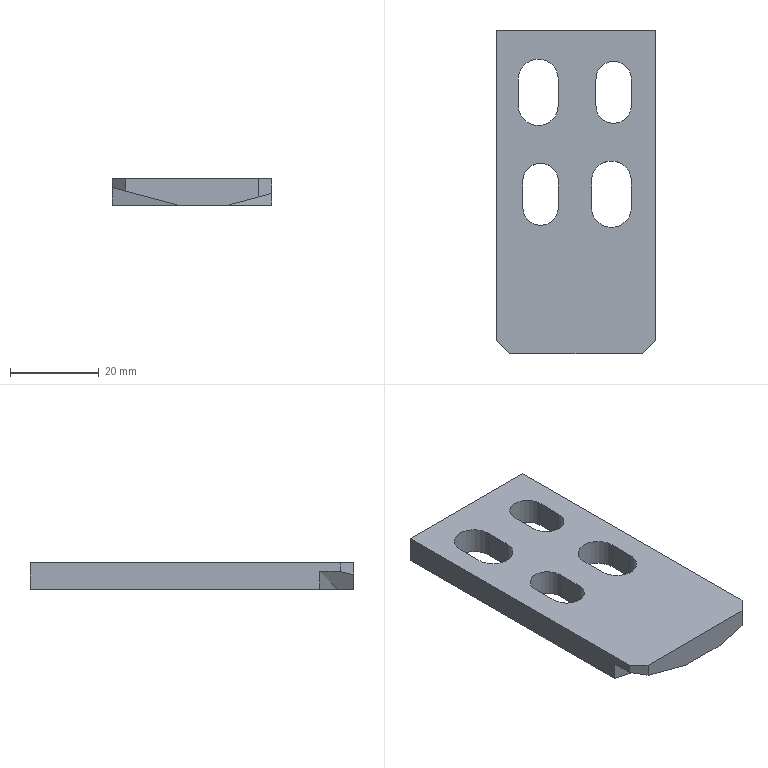Part | STEP file | gslz 2016.10.28-13_id1738_x_t | 1 solid | 29 faces | box 36 x 73 x 6 mm | volume 12869 mm3 | plane 21 | cylinder 8 | commonest cylinder face diameters 8 x4 9 x4